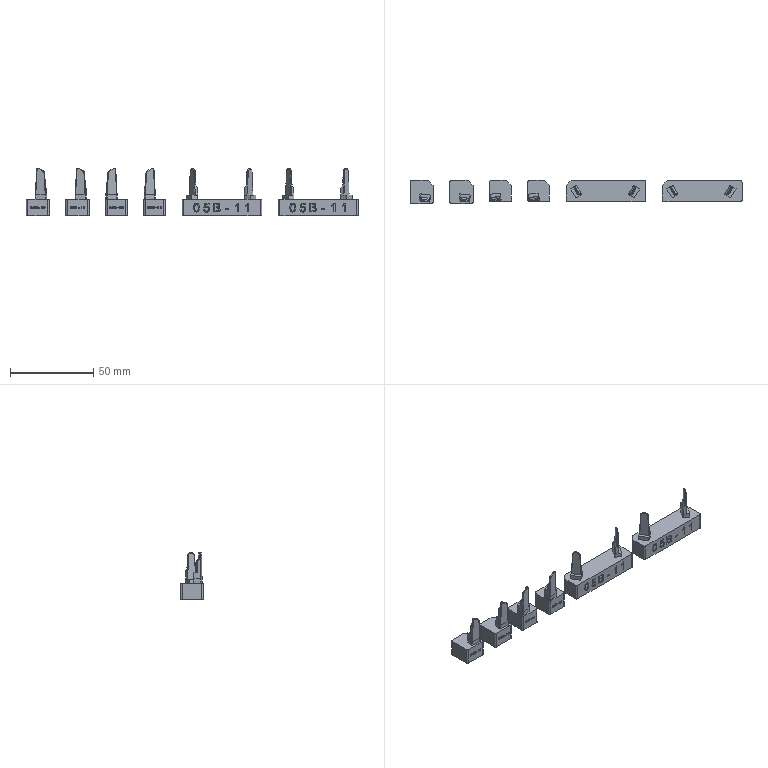NC program | NX | posted with a generic post | part box 200 x 14 x 28.763 mm
Lines 67505 to 68265 of 209396:
(ZLEVEL_PROFILE_CLIMB_0_0 , TOOL : D8-0.075)
N134924 M6
N134926 G53
N134928 G17 G0 G90 X-99.216 Y-6.553 S10000 M3
N134930 G43 Z30.025 H0
N134932 Z-0.325
N134934 G94 G3 X-96.99 Y-4.48 R2.355 F4000.
N134936 G1 X-96.975 Y-4.354
N134938 G2 X-94.191 Y-0.942 R4.146
N134940 X-92.241 Y-0.713 R4.659
N134942 X-90.292 Y-1.287 R4.883
N134944 X-88.144 Y-5.517 R4.162
N134946 X-91.158 Y-9.141 R4.167
N134948 X-93.108 Y-9.281 R4.852
N134950 X-95.058 Y-8.609 R4.771
N134952 X-97.005 Y-4.606 R4.152
N134954 G1 X-96.99 Y-4.48
N134956 X-96.979 Y-4.373 Z-0.326
N134958 X-96.966 Y-4.266 Z-0.327
N134960 X-96.951 Y-4.16 Z-0.328
N134962 X-96.933 Y-4.054 Z-0.329
N134964 X-96.912 Y-3.948 Z-0.33
N134966 X-96.888 Y-3.843 Z-0.331
N134968 X-96.863 Y-3.739 Z-0.332
N134970 X-96.833 Y-3.635 Z-0.333
N134972 X-96.802 Y-3.532
N134974 X-96.766 Y-3.43 Z-0.334
N134976 X-96.729 Y-3.328 Z-0.335
N134978 X-96.689 Y-3.228 Z-0.336
N134980 X-96.647 Y-3.129 Z-0.337
N134982 X-96.601 Y-3.031 Z-0.338
N134984 X-96.555 Y-2.934 Z-0.339
N134986 X-96.503 Y-2.839 Z-0.34
N134988 X-96.451 Y-2.744 Z-0.341
N134990 X-96.395 Y-2.651 Z-0.342
N134992 X-96.338 Y-2.559 Z-0.343
N134994 X-96.276 Y-2.47 Z-0.344
N134996 X-96.247 Y-2.425
N134998 X-96.215 Y-2.381 Z-0.345
N135000 X-96.183 Y-2.338
N135002 X-96.149 Y-2.296 Z-0.346
N135004 X-96.083 Y-2.21 Z-0.347
N135006 X-96.012 Y-2.128 Z-0.348
N135008 X-95.978 Y-2.086
N135010 X-95.942 Y-2.045
N135012 X-95.905 Y-2.005 Z-0.349
N135014 X-95.867 Y-1.967
N135016 X-95.83 Y-1.927 Z-0.35
N135018 X-95.792 Y-1.889
N135020 X-95.753 Y-1.851 Z-0.351
N135022 X-95.713 Y-1.815
N135024 X-95.674 Y-1.777 Z-0.352
N135026 X-95.634 Y-1.74
N135028 X-95.594 Y-1.704 Z-0.353
N135030 X-95.551 Y-1.67
N135032 X-95.511 Y-1.634 Z-0.354
N135034 X-95.469 Y-1.6
N135036 X-95.427 Y-1.566 Z-0.355
N135038 X-95.382 Y-1.535
N135040 X-95.34 Y-1.501
N135042 X-95.297 Y-1.469 Z-0.356
N135044 X-95.252 Y-1.438
N135046 X-95.207 Y-1.408 Z-0.357
N135048 X-95.117 Y-1.347 Z-0.358
N135050 X-95.025 Y-1.291 Z-0.359
N135052 X-94.932 Y-1.234 Z-0.36
N135054 X-94.837 Y-1.183 Z-0.361
N135056 X-94.741 Y-1.132 Z-0.362
N135058 X-94.643 Y-1.085 Z-0.363
N135060 X-94.545 Y-1.039
N135062 X-94.445 Y-0.997 Z-0.364
N135064 X-94.345 Y-0.956 Z-0.365
N135066 X-94.243 Y-0.919 Z-0.366
N135068 X-94.14 Y-0.883 Z-0.367
N135070 X-94.037 Y-0.851 Z-0.368
N135072 X-93.933 Y-0.822 Z-0.369
N135074 X-93.828 Y-0.794 Z-0.37
N135076 X-93.722 Y-0.769 Z-0.371
N135078 X-93.616 Y-0.748 Z-0.372
N135080 X-93.51 Y-0.728 Z-0.373
N135082 X-93.403 Y-0.711 Z-0.374
N135084 X-93.295 Y-0.697 Z-0.375
N135086 X-93.188 Y-0.686 Z-0.376
N135088 X-93.08 Y-0.677 Z-0.377
N135090 X-92.972 Y-0.67 Z-0.378
N135092 X-92.864 Y-0.666
N135094 X-92.756 Y-0.664 Z-0.379
N135096 X-92.647 Z-0.38
N135098 X-92.539 Y-0.667 Z-0.381
N135100 X-92.431 Y-0.672 Z-0.382
N135102 X-92.324 Y-0.679 Z-0.383
N135104 X-92.216 Y-0.688 Z-0.384
N135106 X-92.109 Y-0.699 Z-0.385
N135108 X-92.002 Y-0.712 Z-0.386
N135110 X-91.895 Y-0.727 Z-0.387
N135112 X-91.788 Y-0.742 Z-0.388
N135114 X-91.681 Y-0.761 Z-0.389
N135116 X-91.575 Y-0.78 Z-0.39
N135118 X-91.469 Y-0.803 Z-0.391
N135120 X-91.363 Y-0.827 Z-0.392
N135122 X-91.259 Y-0.854 Z-0.393
N135124 X-91.154 Y-0.882
N135126 X-91.05 Y-0.914 Z-0.394
N135128 X-90.947 Y-0.946 Z-0.395
N135130 X-90.845 Y-0.982 Z-0.396
N135132 X-90.742 Y-1.019 Z-0.397
N135134 X-90.642 Y-1.06 Z-0.398
N135136 X-90.542 Y-1.101 Z-0.399
N135138 X-90.443 Y-1.147 Z-0.4
N135140 X-90.345 Y-1.193 Z-0.401
N135142 X-90.249 Y-1.244 Z-0.402
N135144 X-90.152 Y-1.295 Z-0.403
N135146 X-90.058 Y-1.35 Z-0.404
N135148 X-89.964 Y-1.406 Z-0.405
N135150 X-89.873 Y-1.466 Z-0.406
N135152 X-89.826 Y-1.494
N135154 X-89.781 Y-1.525 Z-0.407
N135156 X-89.736 Y-1.557
N135158 X-89.693 Y-1.59 Z-0.408
N135160 X-89.604 Y-1.654
N135162 X-89.519 Y-1.722 Z-0.409
N135164 X-89.433 Y-1.791 Z-0.41
N135166 X-89.351 Y-1.864 Z-0.411
N135168 X-89.27 Y-1.937 Z-0.412
N135170 X-89.191 Y-2.013 Z-0.413
N135172 X-89.113 Y-2.091 Z-0.414
N135174 X-89.038 Y-2.172 Z-0.415
N135176 X-88.964 Y-2.253 Z-0.416
N135178 X-88.893 Y-2.338 Z-0.417
N135180 X-88.825 Y-2.424 Z-0.418
N135182 X-88.756 Y-2.511 Z-0.419
N135184 X-88.692 Y-2.601 Z-0.42
N135186 X-88.628 Y-2.691 Z-0.421
N135188 X-88.568 Y-2.784 Z-0.422
N135190 X-88.51 Y-2.878 Z-0.423
N135192 X-88.454 Y-2.974
N135194 X-88.401 Y-3.072 Z-0.424
N135196 X-88.35 Y-3.17 Z-0.425
N135198 X-88.302 Y-3.271 Z-0.426
N135200 X-88.256 Y-3.372 Z-0.427
N135202 X-88.214 Y-3.475 Z-0.428
N135204 X-88.174 Y-3.579 Z-0.429
N135206 X-88.137 Y-3.684 Z-0.43
N135208 X-88.102 Y-3.791 Z-0.431
N135210 X-88.07 Y-3.898 Z-0.432
N135212 X-88.041 Y-4.006 Z-0.433
N135214 X-88.016 Y-4.114 Z-0.434
N135216 X-87.993 Y-4.224 Z-0.435
N135218 X-87.973 Y-4.334 Z-0.436
N135220 X-87.956 Y-4.445 Z-0.437
N135222 X-87.942 Y-4.556 Z-0.438
N135224 G2 X-87.96 Y-5.517 R4.116
N135226 X-90.075 Y-8.792 R4.156
N135228 X-92.025 Y-9.362 R4.534
N135230 X-93.108 Y-9.32 R5.811
N135232 X-94.408 Y-9.017 R5.231
N135234 X-96.573 Y-7.237 R4.302
N135236 X-97.154 Y-4.592 R4.12
N135238 G1 X-97.138 Y-4.462
N135240 X-97.128 Y-4.368
N135242 X-97.116 Y-4.273 Z-0.439
N135244 X-97.104 Y-4.178 Z-0.44
N135246 X-97.088 Y-4.084 Z-0.441
N135248 X-97.071 Y-3.99 Z-0.442
N135250 X-97.051 Y-3.897 Z-0.443
N135252 X-97.03 Y-3.804
N135254 X-97.006 Y-3.711 Z-0.444
N135256 X-96.98 Y-3.619 Z-0.445
N135258 X-96.951 Y-3.528 Z-0.446
N135260 X-96.921 Y-3.437 Z-0.447
N135262 X-96.888 Y-3.348 Z-0.448
N135264 G2 X-94.999 Y-1.186 R4.169
N135266 X-93.022 Y-0.643 R4.427
N135268 X-92.025 Y-0.696 R5.788
N135270 X-90.942 Y-0.924 R5.723
N135272 X-88.992 Y-2.17 R4.508
N135274 X-87.944 Y-5.517 R4.135
N135276 X-90.075 Y-8.802 R4.157
N135278 X-92.241 Y-9.373 R4.549
N135280 X-93.108 Y-9.321 R6.107
N135282 X-94.191 Y-9.097 R5.446
N135284 X-96.357 Y-7.572 R4.345
N135286 X-97.164 Y-4.588 R4.168
N135288 G1 X-97.149 Y-4.461
N135290 X-97.138 Y-4.363
N135292 X-97.126 Y-4.265 Z-0.449
N135294 X-97.113 Y-4.167 Z-0.45
N135296 X-97.096 Y-4.07 Z-0.451
N135298 X-97.078 Y-3.973 Z-0.452
N135300 X-97.057 Y-3.877 Z-0.453
N135302 X-97.034 Y-3.781 Z-0.454
N135304 X-97.009 Y-3.685
N135306 X-96.981 Y-3.59 Z-0.455
N135308 X-96.951 Y-3.496 Z-0.456
N135310 X-96.92 Y-3.403 Z-0.457
N135312 X-96.885 Y-3.31 Z-0.458
N135314 X-96.849 Y-3.218 Z-0.459
N135316 X-96.81 Y-3.127 Z-0.46
N135318 X-96.769 Y-3.037
N135320 X-96.726 Y-2.948 Z-0.461
N135322 X-96.681 Y-2.86 Z-0.462
N135324 X-96.632 Y-2.773 Z-0.463
N135326 G2 X-94.841 Y-1.089 R4.184
N135328 G1 X-94.7 Y-1.025
N135330 G2 X-93.052 Y-0.639 R4.365
N135332 X-92.025 Y-0.694 R5.812
N135334 X-91.039 Y-0.888 R5.745
N135336 X-88.993 Y-2.146 R4.513
N135338 X-87.919 Y-5.517 R4.135
N135340 X-90.075 Y-8.819 R4.159
N135342 X-92.458 Y-9.376 R4.621
N135344 X-93.541 Y-9.262 R9.089
N135346 X-94.624 Y-8.943 R4.782
N135348 X-96.452 Y-7.464 R4.323
N135350 X-97.18 Y-4.586 R4.169
N135352 G1 X-97.165 Y-4.459
N135354 X-97.153 Y-4.352 Z-0.464
N135356 X-97.14 Y-4.245 Z-0.465
N135358 X-97.124 Y-4.138 Z-0.466
N135360 X-97.105 Y-4.031 Z-0.467
N135362 X-97.084 Y-3.925 Z-0.468
N135364 X-97.06 Y-3.82 Z-0.469
N135366 X-97.033 Y-3.715 Z-0.47
N135368 X-97.004 Y-3.611 Z-0.471
N135370 X-96.971 Y-3.507
N135372 X-96.937 Y-3.405 Z-0.472
N135374 X-96.899 Y-3.303 Z-0.473
N135376 X-96.859 Y-3.203 Z-0.474
N135378 X-96.816 Y-3.103 Z-0.475
N135380 X-96.77 Y-3.005 Z-0.476
N135382 X-96.722 Y-2.907 Z-0.477
N135384 X-96.672 Y-2.812 Z-0.478
N135386 X-96.619 Y-2.717 Z-0.479
N135388 X-96.562 Y-2.624 Z-0.48
N135390 G2 X-94.841 Y-1.076 R4.186
N135392 X-92.891 Y-0.631 R4.436
N135394 X-92.025 Y-0.694 R6.014
N135396 X-91.098 Y-0.865 R6.092
N135398 X-88.992 Y-2.121 R4.558
N135400 X-87.891 Y-5.517 R4.135
N135402 X-90.292 Y-8.947 R4.168
N135404 X-92.458 Y-9.38 R4.648
N135406 X-93.541 Y-9.265 R10.151
N135408 X-94.557 Y-8.979 R4.854
N135410 X-96.141 Y-7.875 R4.357
N135412 X-97.197 Y-4.585 R4.173
N135414 G1 X-97.182 Y-4.457
N135416 X-97.171 Y-4.36 Z-0.481
N135418 X-97.159 Y-4.263 Z-0.482
N135420 X-97.146 Y-4.166 Z-0.483
N135422 X-97.129 Y-4.069
N135424 X-97.111 Y-3.973 Z-0.484
N135426 X-97.091 Y-3.877 Z-0.485
N135428 X-97.069 Y-3.782 Z-0.486
N135430 X-97.044 Y-3.687 Z-0.487
N135432 X-97.016 Y-3.593 Z-0.488
N135434 X-96.986 Y-3.499 Z-0.489
N135436 X-96.955 Y-3.406
N135438 X-96.921 Y-3.314 Z-0.49
N135440 X-96.885 Y-3.223 Z-0.491
N135442 X-96.847 Y-3.132 Z-0.492
N135444 X-96.806 Y-3.043 Z-0.493
N135446 X-96.763 Y-2.955 Z-0.494
N135448 X-96.72 Y-2.867 Z-0.495
N135450 X-96.672 Y-2.781
N135452 X-96.624 Y-2.695 Z-0.496
N135454 X-96.572 Y-2.612 Z-0.497
N135456 G2 X-94.841 Y-1.065 R4.189
N135458 X-92.891 Y-0.626 R4.434
N135460 X-92.025 Y-0.694 R6.278
N135462 X-91.081 Y-0.865 R6.111
N135464 X-88.992 Y-2.095 R4.573
N135466 X-87.863 Y-5.517 R4.137
N135468 X-90.292 Y-8.963 R4.171
N135470 X-92.458 Y-9.383 R4.693
N135472 X-93.541 Y-9.267 R12.042
N135474 X-95.03 Y-8.763 R4.686
N135476 X-96.951 Y-6.599 R4.255
N135478 X-97.213 Y-4.583 R4.209
N135480 G1 X-97.198 Y-4.455
N135482 X-97.187 Y-4.357 Z-0.498
N135484 X-97.175 Y-4.26 Z-0.499
N135486 X-97.161 Y-4.162 Z-0.5
N135488 X-97.145 Y-4.065 Z-0.501
N135490 X-97.126 Y-3.968
N135492 X-97.106 Y-3.872 Z-0.502
N135494 X-97.083 Y-3.776 Z-0.503
N135496 X-97.058 Y-3.68 Z-0.504
N135498 X-97.03 Y-3.586 Z-0.505
N135500 X-97. Y-3.492 Z-0.506
N135502 X-96.968 Y-3.398 Z-0.507
N135504 X-96.934 Y-3.306
N135506 X-96.898 Y-3.214 Z-0.508
N135508 X-96.859 Y-3.123 Z-0.509
N135510 X-96.818 Y-3.033 Z-0.51
N135512 X-96.775 Y-2.944 Z-0.511
N135514 X-96.73 Y-2.856 Z-0.512
N135516 X-96.683 Y-2.769 Z-0.513
N135518 X-96.634 Y-2.683
N135520 X-96.581 Y-2.6 Z-0.514
N135522 G2 X-94.841 Y-1.053 R4.201
N135524 G1 X-94.728 Y-1.002
N135526 G2 X-93.334 Y-0.641 R4.361
N135528 X-92.397 Y-0.649 R4.869
N135530 X-91.557 Y-0.757 R18.24
N135532 X-89.502 Y-1.623 R4.741
N135534 X-87.835 Y-5.517 R4.17
N135536 X-90.508 Y-9.071 R4.181
N135538 X-92.675 Y-9.371 R4.787
N135540 X-93.325 Y-9.299 R31.318
N135542 X-94.408 Y-9.049 R4.963
N135544 X-96.574 Y-7.357 R4.316
N135546 X-97.228 Y-4.581 R4.188
N135548 G1 X-97.213 Y-4.453
N135550 X-97.202 Y-4.354 Z-0.515
N135552 X-97.19 Y-4.256 Z-0.516
N135554 X-97.176 Y-4.157 Z-0.517
N135556 X-97.159 Y-4.059 Z-0.518
N135558 X-97.14 Y-3.961 Z-0.519
N135560 X-97.12 Y-3.863
N135562 X-97.096 Y-3.766 Z-0.52
N135564 X-97.07 Y-3.67 Z-0.521
N135566 X-97.042 Y-3.574 Z-0.522
N135568 X-97.012 Y-3.479 Z-0.523
N135570 X-96.979 Y-3.385 Z-0.524
N135572 X-96.944 Y-3.291 Z-0.525
N135574 X-96.907 Y-3.198 Z-0.526
N135576 X-96.868 Y-3.107
N135578 X-96.826 Y-3.016 Z-0.527
N135580 X-96.782 Y-2.926 Z-0.528
N135582 X-96.737 Y-2.837 Z-0.529
N135584 X-96.688 Y-2.75 Z-0.53
N135586 X-96.638 Y-2.663 Z-0.531
N135588 X-96.587 Y-2.577 Z-0.532
N135590 G2 X-95.722 Y-1.603 R4.157
N135592 X-93.32 Y-0.634 R4.329
N135594 X-92.393 Y-0.649 R4.897
N135596 X-91.547 Y-0.757 R23.984
N135598 X-89.425 Y-1.664 R4.723
N135600 X-87.807 Y-5.517 R4.16
N135602 X-90.508 Y-9.086 R4.194
N135604 X-92.675 Y-9.372 R4.818
N135606 X-93.541 Y-9.271 R26.123
N135608 X-94.841 Y-8.876 R4.703
N135610 X-96.888 Y-6.815 R4.271
N135612 X-97.243 Y-4.579 R4.183
N135614 G1 X-97.228 Y-4.452
N135616 X-97.216 Y-4.347 Z-0.533
N135618 X-97.203 Y-4.242
N135620 X-97.188 Y-4.137 Z-0.534
N135622 X-97.17 Y-4.033 Z-0.535
N135624 X-97.15 Y-3.929 Z-0.536
N135626 X-97.126 Y-3.826 Z-0.537
N135628 X-97.101 Y-3.723 Z-0.538
N135630 X-97.072 Y-3.622 Z-0.539
N135632 X-97.041 Y-3.52 Z-0.54
N135634 X-97.008 Y-3.42 Z-0.541
N135636 X-96.972 Y-3.32 Z-0.542
N135638 X-96.933 Y-3.222 Z-0.543
N135640 X-96.891 Y-3.124 Z-0.544
N135642 X-96.848 Y-3.028 Z-0.545
N135644 X-96.802 Y-2.932
N135646 X-96.753 Y-2.838 Z-0.546
N135648 X-96.702 Y-2.745 Z-0.547
N135650 X-96.649 Y-2.654 Z-0.548
N135652 X-96.593 Y-2.564 Z-0.549
N135654 X-96.534 Y-2.476 Z-0.55
N135656 G2 X-94.408 Y-0.855 R4.208
N135658 X-92.458 Y-0.64 R4.531
N135660 G1 X-92.378 Y-0.649
N135662 X-91.592 Y-0.749
N135664 G2 X-89.454 Y-1.623 R4.775
N135666 X-87.777 Y-5.517 R4.173
N135668 X-89.988 Y-8.864 R4.186
N135670 X-91.375 Y-9.332 R4.527
N135672 X-92.891 Y-9.349 R5.076
N135674 X-93.758 Y-9.235 R10.975
N135676 X-95.433 Y-8.546 R4.521
N135678 X-97.258 Y-4.578 R4.21
N135680 G1 X-97.243 Y-4.45
N135682 X-97.231 Y-4.342 Z-0.551
N135684 X-97.217 Y-4.235 Z-0.552
N135686 X-97.202 Y-4.127 Z-0.553
N135688 X-97.182 Y-4.021 Z-0.554
N135690 X-97.161 Y-3.914 Z-0.555
N135692 X-97.137 Y-3.808 Z-0.556
N135694 X-97.11 Y-3.703 Z-0.557
N135696 X-97.08 Y-3.599 Z-0.558
N135698 X-97.048 Y-3.495 Z-0.559
N135700 X-97.013 Y-3.392 Z-0.56
N135702 X-96.975 Y-3.29
N135704 X-96.935 Y-3.189 Z-0.561
N135706 X-96.891 Y-3.09 Z-0.562
N135708 X-96.846 Y-2.991 Z-0.563
N135710 X-96.797 Y-2.893 Z-0.564
N135712 X-96.746 Y-2.797 Z-0.565
N135714 X-96.693 Y-2.703 Z-0.566
N135716 X-96.637 Y-2.609 Z-0.567
N135718 X-96.579 Y-2.517 Z-0.568
N135720 X-96.518 Y-2.427 Z-0.569
N135722 X-96.456 Y-2.338 Z-0.57
N135724 X-96.39 Y-2.251 Z-0.571
N135726 X-96.323 Y-2.166 Z-0.572
N135728 X-96.253 Y-2.082 Z-0.573
N135730 X-96.181 Y-2. Z-0.574
N135732 X-96.107 Y-1.921 Z-0.575
N135734 X-96.031 Y-1.843 Z-0.576
N135736 X-95.953 Y-1.767 Z-0.577
N135738 G2 X-94.624 Y-0.923 R4.206
N135740 X-92.458 Y-0.639 R4.48
N135742 G1 X-91.592 Y-0.748
N135744 X-91.528 Y-0.757
N135746 G2 X-89.739 Y-1.406 R4.839
N135748 X-87.752 Y-4.327 R4.24
N135750 X-87.846 Y-6.186 R4.861
N135752 X-89.919 Y-8.856 R4.168
N135754 X-91.315 Y-9.334 R4.546
N135756 X-92.675 Y-9.374 R4.975
N135758 G1 X-93.47 Y-9.282
N135760 G2 X-95.475 Y-8.532 R4.46
N135762 X-97.279 Y-4.575 R4.208
N135764 G1 X-97.264 Y-4.447
N135766 X-97.252 Y-4.342 Z-0.578
N135768 X-97.238 Y-4.237
N135770 X-97.223 Y-4.133 Z-0.579
N135772 X-97.204 Y-4.029 Z-0.58
N135774 X-97.184 Y-3.925 Z-0.581
N135776 X-97.161 Y-3.821 Z-0.582
N135778 X-97.135 Y-3.719 Z-0.583
N135780 X-97.106 Y-3.617 Z-0.584
N135782 X-97.076 Y-3.515 Z-0.585
N135784 X-97.042 Y-3.415 Z-0.586
N135786 X-97.006 Y-3.315 Z-0.587
N135788 X-96.967 Y-3.217 Z-0.588
N135790 X-96.926 Y-3.119 Z-0.589
N135792 X-96.882 Y-3.022 Z-0.59
N135794 X-96.836 Y-2.927
N135796 X-96.788 Y-2.832 Z-0.591
N135798 X-96.736 Y-2.74 Z-0.592
N135800 X-96.683 Y-2.648 Z-0.593
N135802 X-96.627 Y-2.558 Z-0.594
N135804 X-96.569 Y-2.469 Z-0.595
N135806 X-96.509 Y-2.381 Z-0.596
N135808 X-96.446 Y-2.296 Z-0.597
N135810 X-96.382 Y-2.211 Z-0.598
N135812 X-96.315 Y-2.129 Z-0.599
N135814 X-96.247 Y-2.048 Z-0.6
N135816 X-96.175 Y-1.969 Z-0.601
N135818 X-96.103 Y-1.892 Z-0.602
N135820 X-96.028 Y-1.817
N135822 X-95.951 Y-1.743 Z-0.603
N135824 X-95.873 Y-1.672 Z-0.604
N135826 X-95.792 Y-1.602 Z-0.605
N135828 X-95.71 Y-1.535 Z-0.606
N135830 X-95.627 Y-1.469 Z-0.607
N135832 X-95.541 Y-1.406 Z-0.608
N135834 X-95.455 Y-1.345 Z-0.609
N135836 X-95.366 Y-1.286 Z-0.61
N135838 X-95.277 Y-1.229 Z-0.611
N135840 X-95.185 Y-1.175 Z-0.612
N135842 X-95.093 Y-1.123 Z-0.613
N135844 X-94.999 Y-1.073 Z-0.614
N135846 G2 X-94.608 Y-0.899 R4.214
N135848 X-92.595 Y-0.625 R4.407
N135850 G1 X-92.458 Y-0.639
N135852 X-91.592 Y-0.747
N135854 X-91.516 Y-0.757
N135856 G2 X-89.691 Y-1.406 R4.858
N135858 X-87.893 Y-3.57 R4.283
N135860 X-87.673 Y-5.517 R4.115
N135862 X-90.292 Y-9.067 R4.186
N135864 X-92.458 Y-9.395 R4.771
N135866 G1 X-92.675 Y-9.374
N135868 X-93.541 Y-9.275
N135870 G2 X-95.773 Y-8.33 R4.412
N135872 X-97.305 Y-4.573 R4.206
N135874 G1 X-97.29 Y-4.444
N135876 X-97.278 Y-4.34
N135878 X-97.264 Y-4.236 Z-0.615
N135880 X-97.25 Y-4.132 Z-0.616
N135882 X-97.231 Y-4.029 Z-0.617
N135884 X-97.211 Y-3.926 Z-0.618
N135886 X-97.188 Y-3.824 Z-0.619
N135888 X-97.163 Y-3.722 Z-0.62
N135890 X-97.134 Y-3.621 Z-0.621
N135892 X-97.104 Y-3.52 Z-0.622
N135894 X-97.071 Y-3.421 Z-0.623
N135896 X-97.035 Y-3.322 Z-0.624
N135898 X-96.997 Y-3.224
N135900 X-96.956 Y-3.127 Z-0.625
N135902 X-96.913 Y-3.031 Z-0.626
N135904 X-96.868 Y-2.937 Z-0.627
N135906 X-96.82 Y-2.843 Z-0.628
N135908 X-96.77 Y-2.751 Z-0.629
N135910 X-96.717 Y-2.66 Z-0.63
N135912 X-96.663 Y-2.57 Z-0.631
N135914 X-96.606 Y-2.481 Z-0.632
N135916 X-96.547 Y-2.395 Z-0.633
N135918 X-96.485 Y-2.309 Z-0.634
N135920 X-96.422 Y-2.225 Z-0.635
N135922 X-96.356 Y-2.143
N135924 X-96.288 Y-2.063 Z-0.636
N135926 X-96.219 Y-1.984 Z-0.637
N135928 X-96.147 Y-1.907 Z-0.638
N135930 X-96.074 Y-1.832 Z-0.639
N135932 X-95.998 Y-1.758 Z-0.64
N135934 X-95.921 Y-1.687 Z-0.641
N135936 X-95.842 Y-1.618 Z-0.642
N135938 X-95.761 Y-1.55 Z-0.643
N135940 X-95.679 Y-1.484 Z-0.644
N135942 X-95.595 Y-1.421 Z-0.645
N135944 X-95.509 Y-1.36 Z-0.646
N135946 X-95.422 Y-1.301
N135948 X-95.334 Y-1.244 Z-0.647
N135950 X-95.243 Y-1.19 Z-0.648
N135952 X-95.152 Y-1.137 Z-0.649
N135954 X-95.059 Y-1.088 Z-0.65
N135956 X-94.966 Y-1.039 Z-0.651
N135958 X-94.871 Y-0.995 Z-0.652
N135960 X-94.775 Y-0.951 Z-0.653
N135962 X-94.678 Y-0.91 Z-0.654
N135964 X-94.58 Y-0.871 Z-0.655
N135966 X-94.481 Y-0.836 Z-0.656
N135968 X-94.381 Y-0.802
N135970 X-94.281 Y-0.771 Z-0.657
N135972 X-94.18 Y-0.743 Z-0.658
N135974 X-94.078 Y-0.718 Z-0.659
N135976 X-93.975 Y-0.694 Z-0.66
N135978 X-93.872 Y-0.673 Z-0.661
N135980 G2 X-92.587 Y-0.624 R4.376
N135982 G1 X-92.458 Y-0.638
N135984 X-91.505 Y-0.757
N135986 X-91.375 Y-0.776
N135988 G2 X-89.304 Y-1.623 R4.782
N135990 X-87.596 Y-5.517 R4.175
N135992 X-89.859 Y-8.911 R4.168
N135994 X-91.576 Y-9.401 R4.573
N135996 X-92.595 Y-9.384 R5.231
N135998 G1 X-93.541 Y-9.276
N136000 G2 X-96.05 Y-8.114 R4.351
N136002 X-97.335 Y-4.569 R4.21
N136004 G1 X-97.32 Y-4.441
N136006 X-97.308 Y-4.336 Z-0.662
N136008 X-97.294 Y-4.232 Z-0.663
N136010 X-97.28 Y-4.128 Z-0.664
N136012 X-97.26 Y-4.024 Z-0.665
N136014 X-97.241 Y-3.921 Z-0.666
N136016 X-97.217 Y-3.818 Z-0.667
N136018 X-97.192 Y-3.716 Z-0.668
N136020 X-97.163 Y-3.615
N136022 X-97.133 Y-3.514 Z-0.669
N136024 X-97.099 Y-3.414 Z-0.67
N136026 X-97.064 Y-3.315 Z-0.671
N136028 X-97.025 Y-3.217 Z-0.672
N136030 X-96.984 Y-3.119 Z-0.673
N136032 X-96.941 Y-3.023 Z-0.674
N136034 X-96.896 Y-2.928 Z-0.675
N136036 X-96.847 Y-2.834 Z-0.676
N136038 X-96.797 Y-2.742 Z-0.677
N136040 X-96.744 Y-2.651 Z-0.678
N136042 X-96.689 Y-2.56 Z-0.679
N136044 X-96.632 Y-2.472
N136046 X-96.572 Y-2.385 Z-0.68
N136048 X-96.51 Y-2.299 Z-0.681
N136050 X-96.447 Y-2.215 Z-0.682
N136052 X-96.381 Y-2.133 Z-0.683
N136054 X-96.313 Y-2.052 Z-0.684
N136056 X-96.243 Y-1.973 Z-0.685
N136058 X-96.171 Y-1.896 Z-0.686
N136060 X-96.097 Y-1.821 Z-0.687
N136062 X-96.021 Y-1.747 Z-0.688
N136064 X-95.943 Y-1.676 Z-0.689
N136066 X-95.864 Y-1.606 Z-0.69
N136068 X-95.783 Y-1.538
N136070 X-95.7 Y-1.473 Z-0.691
N136072 X-95.615 Y-1.41 Z-0.692
N136074 X-95.53 Y-1.348 Z-0.693
N136076 X-95.442 Y-1.29 Z-0.694
N136078 X-95.354 Y-1.232 Z-0.695
N136080 X-95.263 Y-1.178 Z-0.696
N136082 X-95.172 Y-1.125 Z-0.697
N136084 X-95.078 Y-1.076 Z-0.698
N136086 X-94.984 Y-1.027 Z-0.699
N136088 X-94.889 Y-0.982 Z-0.7
N136090 X-94.793 Y-0.939 Z-0.701
N136092 X-94.695 Y-0.899
N136094 X-94.597 Y-0.861 Z-0.702
N136096 X-94.497 Y-0.826 Z-0.703
N136098 X-94.397 Y-0.792 Z-0.704
N136100 X-94.296 Y-0.761 Z-0.705
N136102 X-94.194 Y-0.733 Z-0.706
N136104 X-94.092 Y-0.708 Z-0.707
N136106 X-93.989 Y-0.684 Z-0.708
N136108 X-93.886 Y-0.664 Z-0.709
N136110 X-93.782 Y-0.646 Z-0.71
N136112 X-93.677 Y-0.63 Z-0.711
N136114 X-93.573 Y-0.617 Z-0.712
N136116 X-93.468 Y-0.607
N136118 X-93.362 Y-0.6 Z-0.713
N136120 X-93.257 Y-0.595 Z-0.714
N136122 X-93.152 Y-0.593 Z-0.715
N136124 X-93.046 Y-0.592 Z-0.716
N136126 X-92.941 Y-0.594 Z-0.717
N136128 X-92.836 Y-0.6 Z-0.718
N136130 X-92.731 Y-0.607 Z-0.719
N136132 X-92.626 Y-0.618 Z-0.72
N136134 X-92.598 Y-0.621
N136136 X-92.458 Y-0.638
N136138 X-91.5 Y-0.757
N136140 X-91.375 Y-0.773
N136142 G2 X-89.961 Y-1.19 R4.951
N136144 X-88.51 Y-2.272 R4.489
N136146 X-87.5 Y-5.517 R4.134
N136148 X-89.859 Y-8.971 R4.18
N136150 X-91.592 Y-9.421 R4.658
N136152 X-92.458 Y-9.4 R5.238
N136154 G1 X-93.541 Y-9.277
N136156 X-93.758 Y-9.248
N136158 G2 X-96.141 Y-8.059 R4.321
N136160 X-97.366 Y-4.567 R4.207
N136162 G1 X-97.368 Y-4.566
N136164 X-97.353 Y-4.437
N136166 X-97.341 Y-4.331 Z-0.721
N136168 X-97.326 Y-4.225 Z-0.722
N136170 X-97.311 Y-4.12 Z-0.723
N136172 X-97.292 Y-4.015 Z-0.724
N136174 X-97.272 Y-3.911
N136176 X-97.248 Y-3.807 Z-0.725
N136178 X-97.222 Y-3.703 Z-0.726
N136180 X-97.192 Y-3.601 Z-0.727
N136182 X-97.162 Y-3.499 Z-0.728
N136184 X-97.127 Y-3.398 Z-0.729
N136186 X-97.091 Y-3.298 Z-0.73
N136188 X-97.051 Y-3.199 Z-0.731
N136190 X-97.01 Y-3.1 Z-0.732
N136192 X-96.965 Y-3.003 Z-0.733
N136194 X-96.919 Y-2.907 Z-0.734
N136196 X-96.869 Y-2.813 Z-0.735
N136198 X-96.819 Y-2.719 Z-0.736
N136200 X-96.764 Y-2.627 Z-0.737
N136202 X-96.709 Y-2.536
N136204 X-96.65 Y-2.447 Z-0.738
N136206 X-96.589 Y-2.359 Z-0.739
N136208 X-96.526 Y-2.273 Z-0.74
N136210 X-96.461 Y-2.188 Z-0.741
N136212 X-96.394 Y-2.106 Z-0.742
N136214 X-96.325 Y-2.024 Z-0.743
N136216 X-96.253 Y-1.945 Z-0.744
N136218 X-96.18 Y-1.867 Z-0.745
N136220 X-96.104 Y-1.792 Z-0.746
N136222 X-96.027 Y-1.718 Z-0.747
N136224 X-95.948 Y-1.646 Z-0.748
N136226 X-95.867 Y-1.576 Z-0.749
N136228 X-95.785 Y-1.509 Z-0.75
N136230 X-95.7 Y-1.443 Z-0.751
N136232 X-95.614 Y-1.38
N136234 X-95.527 Y-1.319 Z-0.752
N136236 X-95.438 Y-1.26 Z-0.753
N136238 X-95.347 Y-1.203 Z-0.754
N136240 X-95.255 Y-1.15 Z-0.755
N136242 X-95.162 Y-1.097 Z-0.756
N136244 X-95.067 Y-1.048 Z-0.757
N136246 X-94.972 Y-1. Z-0.758
N136248 X-94.875 Y-0.955 Z-0.759
N136250 X-94.777 Y-0.913 Z-0.76
N136252 X-94.677 Y-0.875 Z-0.761
N136254 X-94.578 Y-0.836 Z-0.762
N136256 X-94.477 Y-0.803 Z-0.763
N136258 X-94.375 Y-0.769 Z-0.764
N136260 X-94.272 Y-0.74
N136262 X-94.169 Y-0.713 Z-0.765
N136264 X-94.066 Y-0.688 Z-0.766
N136266 X-93.961 Y-0.666 Z-0.767
N136268 X-93.856 Y-0.647 Z-0.768
N136270 X-93.751 Y-0.631 Z-0.769
N136272 X-93.645 Y-0.616 Z-0.77
N136274 X-93.539 Y-0.605 Z-0.771
N136276 X-93.432 Y-0.596 Z-0.772
N136278 X-93.326 Y-0.59 Z-0.773
N136280 X-93.219 Y-0.587 Z-0.774
N136282 X-93.113 Y-0.586 Z-0.775
N136284 X-93.006 Y-0.588 Z-0.776
N136286 X-92.9 Y-0.592 Z-0.777
N136288 X-92.793 Y-0.6
N136290 X-92.687 Y-0.609 Z-0.778
N136292 X-92.581 Y-0.622 Z-0.779
N136294 X-92.476 Y-0.635 Z-0.78
N136296 X-92.37 Y-0.648 Z-0.781
N136298 X-92.264 Y-0.661 Z-0.782
N136300 X-92.159 Y-0.674 Z-0.783
N136302 X-91.947 Y-0.701 Z-0.785
N136304 X-91.842 Y-0.714 Z-0.786
N136306 X-91.736 Y-0.727 Z-0.787
N136308 X-91.63 Y-0.74 Z-0.788
N136310 X-91.525 Y-0.754 Z-0.789
N136312 X-91.375 Y-0.772
N136314 X-91.227 Y-0.793
N136316 G2 X-89.126 Y-1.628 R4.778
N136318 X-87.413 Y-5.734 R4.197
N136320 X-89.453 Y-8.825 R4.144
N136322 X-90.906 Y-9.362 R4.56
N136324 X-92.361 Y-9.412 R4.921
N136326 G1 X-93.541 Y-9.277
N136328 X-93.758 Y-9.25
N136330 G2 X-97.137 Y-6.599 R4.256
N136332 X-97.4 Y-4.562 R4.227
N136334 G1 X-97.385 Y-4.433
N136336 X-97.372 Y-4.326 Z-0.79
N136338 X-97.359 Y-4.22
N136340 X-97.343 Y-4.114 Z-0.791
N136342 X-97.324 Y-4.009 Z-0.792
N136344 X-97.303 Y-3.903 Z-0.793
N136346 X-97.279 Y-3.799 Z-0.794
N136348 X-97.252 Y-3.695 Z-0.795
N136350 X-97.223 Y-3.592 Z-0.796
N136352 X-97.191 Y-3.489 Z-0.797
N136354 X-97.157 Y-3.388 Z-0.798
N136356 X-97.12 Y-3.287 Z-0.799
N136358 X-97.08 Y-3.187 Z-0.8
N136360 X-97.038 Y-3.088 Z-0.801
N136362 X-96.993 Y-2.991 Z-0.802
N136364 X-96.946 Y-2.894 Z-0.803
N136366 X-96.896 Y-2.799 Z-0.804
N136368 X-96.844 Y-2.705 Z-0.805
N136370 X-96.79 Y-2.613
N136372 X-96.733 Y-2.521 Z-0.806
N136374 X-96.673 Y-2.432 Z-0.807
N136376 X-96.613 Y-2.344 Z-0.808
N136378 X-96.549 Y-2.257 Z-0.809
N136380 X-96.483 Y-2.172 Z-0.81
N136382 X-96.414 Y-2.09 Z-0.811
N136384 X-96.345 Y-2.007 Z-0.812
N136386 X-96.273 Y-1.928 Z-0.813
N136388 X-96.199 Y-1.85 Z-0.814
N136390 X-96.122 Y-1.775 Z-0.815
N136392 X-96.045 Y-1.7 Z-0.816
N136394 X-95.964 Y-1.629 Z-0.817
N136396 X-95.883 Y-1.559 Z-0.818
N136398 X-95.799 Y-1.492 Z-0.819
N136400 X-95.715 Y-1.425
N136402 X-95.627 Y-1.363 Z-0.82
N136404 X-95.54 Y-1.301 Z-0.821
N136406 X-95.45 Y-1.242 Z-0.822
N136408 X-95.358 Y-1.186 Z-0.823
N136410 X-95.265 Y-1.132 Z-0.824
N136412 X-95.171 Y-1.08 Z-0.825
N136414 X-95.076 Y-1.031 Z-0.826
N136416 X-94.979 Y-0.983 Z-0.827
N136418 X-94.881 Y-0.939 Z-0.828
N136420 X-94.783 Y-0.897 Z-0.829
N136422 X-94.683 Y-0.858 Z-0.83
N136424 X-94.582 Y-0.82 Z-0.831
N136426 X-94.48 Y-0.786 Z-0.832
N136428 X-94.378 Y-0.754 Z-0.833
N136430 X-94.274 Y-0.725 Z-0.834
N136432 X-94.17 Y-0.699
N136434 X-94.065 Y-0.675 Z-0.835
N136436 X-93.96 Y-0.654 Z-0.836
N136438 X-93.854 Y-0.635 Z-0.837